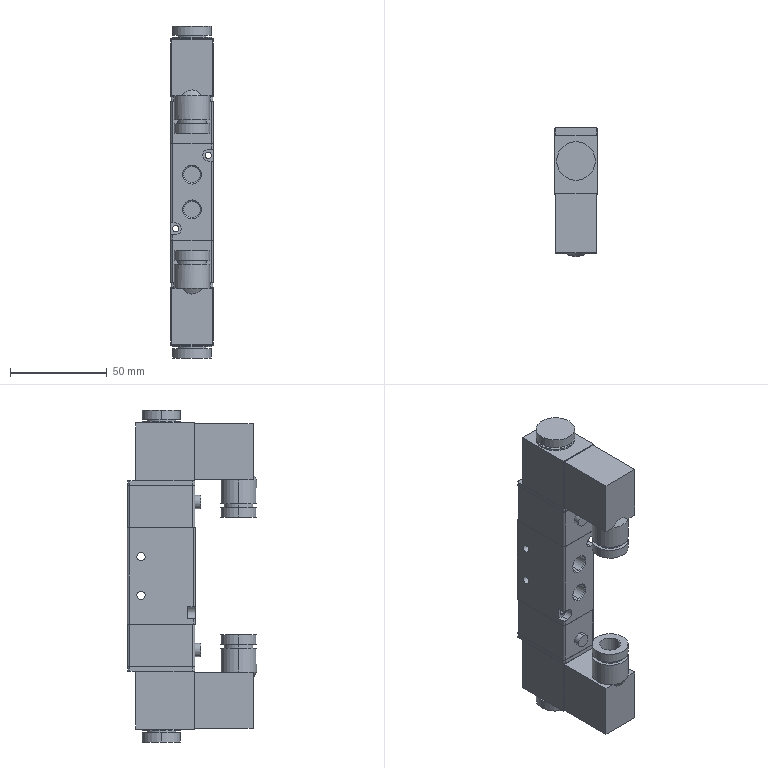Part | STEP file | _4V220-06(By).stp | 1 solid | 165 faces | box 22 x 66.8 x 171.8 mm | volume 158549 mm3 | plane 79 | cylinder 74 | cone 12 | commonest cylinder face diameters 2 x22 8.566 x10 15 x8 18.6 x8 20 x8 3.2 x4